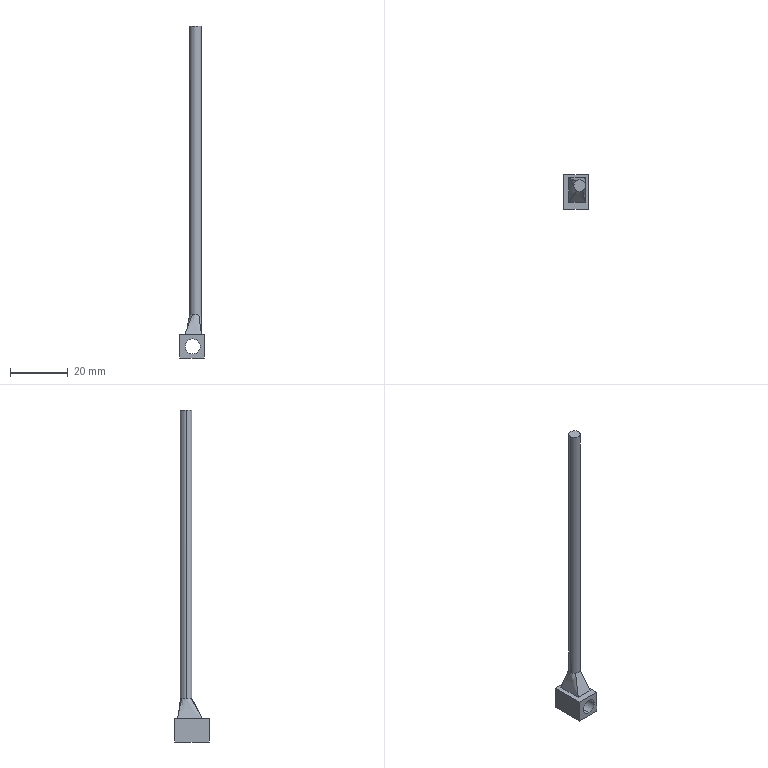Part | SolidWorks | features ICE 4, Blend 1, Extrusion 1 | 1 solid | 15 faces | box 8.5 x 12 x 115 mm | volume 2022 mm3 | plane 7 | cylinder 4 | spline 4 | commonest cylinder face diameters 4 x2 5.2 x2
STEP:
#1=CARTESIAN_POINT('',(-846.11,220.914,0.));
#2=VERTEX_POINT('',#1);
#3=CARTESIAN_POINT('',(-846.999,219.251,0.));
#4=VERTEX_POINT('',#3);
#5=CARTESIAN_POINT('',(-844.999,219.251,0.));
#6=DIRECTION('',(0.,0.,1.));
#7=DIRECTION('',(1.,0.,0.));
#8=AXIS2_PLACEMENT_3D('',#5,#6,#7);
#9=CIRCLE('',#8,2.);
#10=EDGE_CURVE('',#2,#4,#9,.T.);
#11=ORIENTED_EDGE('',*,*,#10,.T.);
#12=CARTESIAN_POINT('',(-846.999,219.251,100.));
#13=VERTEX_POINT('',#12);
#14=CARTESIAN_POINT('',(-846.999,219.251,-7.));
#15=DIRECTION('',(0.,0.,1.));
#16=VECTOR('',#15,1000.);
#17=LINE('',#14,#16);
#18=EDGE_CURVE('',#4,#13,#17,.T.);
#19=ORIENTED_EDGE('',*,*,#18,.T.);
#20=CARTESIAN_POINT('',(-842.999,219.251,100.));
#21=VERTEX_POINT('',#20);
#22=CARTESIAN_POINT('',(-844.999,219.251,100.));
#23=DIRECTION('',(0.,0.,1.));
#24=DIRECTION('',(1.,0.,0.));
#25=AXIS2_PLACEMENT_3D('',#22,#23,#24);
#26=CIRCLE('',#25,2.);
#27=EDGE_CURVE('',#21,#13,#26,.T.);
#28=ORIENTED_EDGE('',*,*,#27,.F.);
#29=CARTESIAN_POINT('',(-842.999,219.256,0.000005697));
#30=VERTEX_POINT('',#29);
#31=CARTESIAN_POINT('',(-842.999,219.251,-7.));
#32=DIRECTION('',(0.,0.,1.));
#33=VECTOR('',#32,1000.);
#34=LINE('',#31,#33);
#35=EDGE_CURVE('',#30,#21,#34,.T.);
#36=ORIENTED_EDGE('',*,*,#35,.F.);
#37=CARTESIAN_POINT('',(-843.888,220.914,0.));
#38=VERTEX_POINT('',#37);
#39=CARTESIAN_POINT('',(-843.888,220.914,0.));
#40=CARTESIAN_POINT('',(-843.866,220.899,0.));
#41=CARTESIAN_POINT('',(-843.84,220.881,-0.0001187));
#42=CARTESIAN_POINT('',(-843.796,220.849,-0.000475));
#43=CARTESIAN_POINT('',(-843.78,220.837,-0.0006234));
#44=CARTESIAN_POINT('',(-843.756,220.817,-0.0008905));
#45=CARTESIAN_POINT('',(-843.747,220.811,-0.000987));
#46=CARTESIAN_POINT('',(-843.73,220.797,-0.001195));
#47=CARTESIAN_POINT('',(-843.722,220.791,-0.001289));
#48=CARTESIAN_POINT('',(-843.671,220.747,-0.001968));
#49=CARTESIAN_POINT('',(-843.637,220.716,-0.0024));
#50=CARTESIAN_POINT('',(-843.598,220.678,-0.002883));
#51=CARTESIAN_POINT('',(-843.586,220.667,-0.003017));
#52=CARTESIAN_POINT('',(-843.572,220.652,-0.003175));
#53=CARTESIAN_POINT('',(-843.565,220.645,-0.003244));
#54=CARTESIAN_POINT('',(-843.558,220.638,-0.003307));
#55=CARTESIAN_POINT('',(-843.556,220.636,-0.00333));
#56=CARTESIAN_POINT('',(-843.554,220.634,-0.003344));
#57=CARTESIAN_POINT('',(-843.554,220.634,-0.003343));
#58=CARTESIAN_POINT('',(-843.526,220.604,-0.003576));
#59=CARTESIAN_POINT('',(-843.5,220.576,-0.003669));
#60=CARTESIAN_POINT('',(-843.453,220.52,-0.003607));
#61=CARTESIAN_POINT('',(-843.432,220.494,-0.003469));
#62=CARTESIAN_POINT('',(-843.388,220.436,-0.002871));
#63=CARTESIAN_POINT('',(-843.356,220.392,-0.002279));
#64=CARTESIAN_POINT('',(-843.32,220.338,-0.00134));
#65=CARTESIAN_POINT('',(-843.302,220.31,-0.0008085));
#66=CARTESIAN_POINT('',(-843.294,220.296,-0.000527));
#67=CARTESIAN_POINT('',(-843.29,220.29,-0.000403));
#68=CARTESIAN_POINT('',(-843.288,220.286,-0.0003196));
#69=CARTESIAN_POINT('',(-843.286,220.283,-0.000257));
#70=CARTESIAN_POINT('',(-843.284,220.28,-0.0001913));
#71=CARTESIAN_POINT('',(-843.282,220.277,-0.0001516));
#72=CARTESIAN_POINT('',(-843.278,220.269,-0.00008074));
#73=CARTESIAN_POINT('',(-843.274,220.262,-0.0000412));
#74=CARTESIAN_POINT('',(-843.266,220.25,0.0000152));
#75=CARTESIAN_POINT('',(-843.262,220.243,0.00001207));
#76=CARTESIAN_POINT('',(-843.252,220.225,-0.0001141));
#77=CARTESIAN_POINT('',(-843.245,220.212,-0.0002929));
#78=CARTESIAN_POINT('',(-843.239,220.201,-0.0005981));
#79=CARTESIAN_POINT('',(-843.235,220.193,-0.0008296));
#80=CARTESIAN_POINT('',(-843.233,220.191,-0.0009036));
#81=CARTESIAN_POINT('',(-843.225,220.175,-0.001502));
#82=CARTESIAN_POINT('',(-843.218,220.162,-0.002265));
#83=CARTESIAN_POINT('',(-843.212,220.148,-0.003443));
#84=CARTESIAN_POINT('',(-843.209,220.143,-0.004009));
#85=CARTESIAN_POINT('',(-843.207,220.139,-0.0044));
#86=CARTESIAN_POINT('',(-843.207,220.139,-0.004427));
#87=CARTESIAN_POINT('',(-843.194,220.113,-0.007893));
#88=CARTESIAN_POINT('',(-843.187,220.097,-0.0151));
#89=CARTESIAN_POINT('',(-843.182,220.086,-0.02857));
#90=CARTESIAN_POINT('',(-843.18,220.081,-0.03853));
#91=CARTESIAN_POINT('',(-843.178,220.077,-0.05581));
#92=CARTESIAN_POINT('',(-843.177,220.075,-0.06443));
#93=CARTESIAN_POINT('',(-843.176,220.074,-0.07044));
#94=CARTESIAN_POINT('',(-843.176,220.073,-0.07513));
#95=CARTESIAN_POINT('',(-843.175,220.072,-0.08376));
#96=CARTESIAN_POINT('',(-843.175,220.07,-0.09594));
#97=CARTESIAN_POINT('',(-843.174,220.068,-0.1133));
#98=CARTESIAN_POINT('',(-843.173,220.068,-0.1215));
#99=CARTESIAN_POINT('',(-843.173,220.067,-0.127));
#100=CARTESIAN_POINT('',(-843.173,220.067,-0.1312));
#101=CARTESIAN_POINT('',(-843.172,220.065,-0.146));
#102=CARTESIAN_POINT('',(-843.171,220.063,-0.17));
#103=CARTESIAN_POINT('',(-843.17,220.06,-0.2052));
#104=CARTESIAN_POINT('',(-843.169,220.058,-0.2246));
#105=CARTESIAN_POINT('',(-843.169,220.058,-0.2334));
#106=CARTESIAN_POINT('',(-843.169,220.057,-0.2392));
#107=CARTESIAN_POINT('',(-843.169,220.057,-0.2441));
#108=CARTESIAN_POINT('',(-843.167,220.054,-0.2815));
#109=CARTESIAN_POINT('',(-843.166,220.05,-0.3372));
#110=CARTESIAN_POINT('',(-843.162,220.042,-0.4498));
#111=CARTESIAN_POINT('',(-843.16,220.037,-0.5133));
#112=CARTESIAN_POINT('',(-843.157,220.031,-0.6002));
#113=CARTESIAN_POINT('',(-843.156,220.028,-0.6402));
#114=CARTESIAN_POINT('',(-843.155,220.026,-0.6674));
#115=CARTESIAN_POINT('',(-843.155,220.025,-0.6825));
#116=CARTESIAN_POINT('',(-843.142,219.994,-1.112));
#117=CARTESIAN_POINT('',(-843.131,219.966,-1.471));
#118=CARTESIAN_POINT('',(-843.118,219.931,-1.921));
#119=CARTESIAN_POINT('',(-843.114,219.92,-2.056));
#120=CARTESIAN_POINT('',(-843.109,219.905,-2.238));
#121=CARTESIAN_POINT('',(-843.107,219.898,-2.323));
#122=CARTESIAN_POINT('',(-843.104,219.891,-2.413));
#123=CARTESIAN_POINT('',(-843.103,219.887,-2.455));
#124=CARTESIAN_POINT('',(-843.102,219.886,-2.476));
#125=CARTESIAN_POINT('',(-843.102,219.885,-2.486));
#126=CARTESIAN_POINT('',(-843.102,219.884,-2.49));
#127=CARTESIAN_POINT('',(-843.102,219.884,-2.493));
#128=CARTESIAN_POINT('',(-843.102,219.884,-2.494));
#129=CARTESIAN_POINT('',(-843.092,219.855,-2.832));
#130=CARTESIAN_POINT('',(-843.084,219.827,-3.146));
#131=CARTESIAN_POINT('',(-843.072,219.786,-3.582));
#132=CARTESIAN_POINT('',(-843.068,219.771,-3.739));
#133=CARTESIAN_POINT('',(-843.064,219.755,-3.897));
#134=CARTESIAN_POINT('',(-843.063,219.752,-3.922));
#135=CARTESIAN_POINT('',(-843.062,219.751,-3.938));
#136=CARTESIAN_POINT('',(-843.062,219.749,-3.953));
#137=CARTESIAN_POINT('',(-843.06,219.742,-4.019));
#138=CARTESIAN_POINT('',(-843.056,219.726,-4.173));
#139=CARTESIAN_POINT('',(-843.042,219.668,-4.711));
#140=CARTESIAN_POINT('',(-843.032,219.617,-5.122));
#141=CARTESIAN_POINT('',(-843.022,219.557,-5.539));
#142=CARTESIAN_POINT('',(-843.018,219.528,-5.729));
#143=CARTESIAN_POINT('',(-843.014,219.495,-5.916));
#144=CARTESIAN_POINT('',(-843.012,219.479,-6.002));
#145=CARTESIAN_POINT('',(-843.011,219.471,-6.043));
#146=CARTESIAN_POINT('',(-843.011,219.467,-6.063));
#147=CARTESIAN_POINT('',(-843.01,219.465,-6.073));
#148=CARTESIAN_POINT('',(-843.01,219.464,-6.077));
#149=CARTESIAN_POINT('',(-843.01,219.463,-6.08));
#150=CARTESIAN_POINT('',(-843.01,219.463,-6.079));
#151=CARTESIAN_POINT('',(-843.008,219.441,-6.187));
#152=CARTESIAN_POINT('',(-843.006,219.42,-6.275));
#153=CARTESIAN_POINT('',(-843.004,219.39,-6.384));
#154=CARTESIAN_POINT('',(-843.003,219.375,-6.432));
#155=CARTESIAN_POINT('',(-843.002,219.358,-6.478));
#156=CARTESIAN_POINT('',(-843.001,219.349,-6.499));
#157=CARTESIAN_POINT('',(-843.001,219.345,-6.508));
#158=CARTESIAN_POINT('',(-843.001,219.343,-6.513));
#159=CARTESIAN_POINT('',(-843.001,219.342,-6.515));
#160=CARTESIAN_POINT('',(-843.001,219.342,-6.516));
#161=CARTESIAN_POINT('',(-843.001,219.342,-6.516));
#162=CARTESIAN_POINT('',(-843.,219.315,-6.572));
#163=CARTESIAN_POINT('',(-842.999,219.291,-6.599));
#164=CARTESIAN_POINT('',(-842.999,219.256,-6.597));
#165=CARTESIAN_POINT('',(-842.999,219.239,-6.586));
#166=CARTESIAN_POINT('',(-842.999,219.22,-6.555));
#167=CARTESIAN_POINT('',(-842.999,219.211,-6.535));
#168=CARTESIAN_POINT('',(-842.999,219.207,-6.525));
#169=CARTESIAN_POINT('',(-843.,219.205,-6.518));
#170=CARTESIAN_POINT('',(-843.,219.203,-6.513));
#171=CARTESIAN_POINT('',(-843.,219.193,-6.486));
#172=CARTESIAN_POINT('',(-843.,219.18,-6.44));
#173=CARTESIAN_POINT('',(-843.001,219.165,-6.371));
#174=CARTESIAN_POINT('',(-843.001,219.158,-6.333));
#175=CARTESIAN_POINT('',(-843.001,219.154,-6.313));
#176=CARTESIAN_POINT('',(-843.001,219.153,-6.304));
#177=CARTESIAN_POINT('',(-843.001,219.152,-6.298));
#178=CARTESIAN_POINT('',(-843.002,219.151,-6.294));
#179=CARTESIAN_POINT('',(-843.002,219.135,-6.197));
#180=CARTESIAN_POINT('',(-843.003,219.121,-6.075));
#181=CARTESIAN_POINT('',(-843.005,219.101,-5.851));
#182=CARTESIAN_POINT('',(-843.005,219.092,-5.728));
#183=CARTESIAN_POINT('',(-843.006,219.083,-5.568));
#184=CARTESIAN_POINT('',(-843.006,219.078,-5.483));
#185=CARTESIAN_POINT('',(-843.007,219.076,-5.439));
#186=CARTESIAN_POINT('',(-843.007,219.075,-5.417));
#187=CARTESIAN_POINT('',(-843.007,219.075,-5.408));
#188=CARTESIAN_POINT('',(-843.007,219.075,-5.401));
#189=CARTESIAN_POINT('',(-843.007,219.074,-5.397));
#190=CARTESIAN_POINT('',(-843.007,219.069,-5.278));
#191=CARTESIAN_POINT('',(-843.008,219.065,-5.145));
#192=CARTESIAN_POINT('',(-843.008,219.059,-4.92));
#193=CARTESIAN_POINT('',(-843.008,219.057,-4.801));
#194=CARTESIAN_POINT('',(-843.009,219.055,-4.652));
#195=CARTESIAN_POINT('',(-843.009,219.054,-4.575));
#196=CARTESIAN_POINT('',(-843.009,219.054,-4.535));
#197=CARTESIAN_POINT('',(-843.009,219.054,-4.515));
#198=CARTESIAN_POINT('',(-843.009,219.054,-4.507));
#199=CARTESIAN_POINT('',(-843.009,219.054,-4.501));
#200=CARTESIAN_POINT('',(-843.009,219.054,-4.497));
#201=CARTESIAN_POINT('',(-843.009,219.053,-4.402));
#202=CARTESIAN_POINT('',(-843.009,219.053,-4.28));
#203=CARTESIAN_POINT('',(-843.009,219.054,-4.055));
#204=CARTESIAN_POINT('',(-843.009,219.054,-3.973));
#205=CARTESIAN_POINT('',(-843.009,219.056,-3.839));
#206=CARTESIAN_POINT('',(-843.008,219.057,-3.769));
#207=CARTESIAN_POINT('',(-843.008,219.058,-3.696));
#208=CARTESIAN_POINT('',(-843.008,219.059,-3.646));
#209=CARTESIAN_POINT('',(-843.008,219.059,-3.619));
#210=CARTESIAN_POINT('',(-843.008,219.067,-3.208));
#211=CARTESIAN_POINT('',(-843.006,219.078,-2.864));
#212=CARTESIAN_POINT('',(-843.005,219.096,-2.414));
#213=CARTESIAN_POINT('',(-843.005,219.102,-2.275));
#214=CARTESIAN_POINT('',(-843.004,219.112,-2.083));
#215=CARTESIAN_POINT('',(-843.004,219.117,-1.991));
#216=CARTESIAN_POINT('',(-843.003,219.122,-1.891));
#217=CARTESIAN_POINT('',(-843.003,219.125,-1.842));
#218=CARTESIAN_POINT('',(-843.003,219.126,-1.819));
#219=CARTESIAN_POINT('',(-843.003,219.127,-1.809));
#220=CARTESIAN_POINT('',(-843.003,219.127,-1.802));
#221=CARTESIAN_POINT('',(-843.003,219.127,-1.8));
#222=CARTESIAN_POINT('',(-843.001,219.161,-1.196));
#223=CARTESIAN_POINT('',(-842.999,219.205,-0.5978));
#224=CARTESIAN_POINT('',(-842.999,219.256,0.000005697));
#225=B_SPLINE_CURVE_WITH_KNOTS('',3,(#39,#40,#41,#42,#43,#44,#45,#46,#47,#48,#49,#50,#51,#52,#53,#54,#55,#56,#57,#58,#59,#60,#61,#62,#63,#64,#65,#66,#67,#68,#69,#70,#71,#72,#73,#74,#75,#76,#77,#78,#79,#80,#81,#82,#83,#84,#85,#86,#87,#88,#89,#90,#91,#92,#93,#94,#95,#96,#97,#98,#99,#100,#101,#102,#103,#104,#105,#106,#107,#108,#109,#110,#111,#112,#113,#114,#115,#116,#117,#118,#119,#120,#121,#122,#123,#124,#125,#126,#127,#128,#129,#130,#131,#132,#133,#134,#135,#136,#137,#138,#139,#140,#141,#142,#143,#144,#145,#146,#147,#148,#149,#150,#151,#152,#153,#154,#155,#156,#157,#158,#159,#160,#161,#162,#163,#164,#165,#166,#167,#168,#169,#170,#171,#172,#173,#174,#175,#176,#177,#178,#179,#180,#181,#182,#183,#184,#185,#186,#187,#188,#189,#190,#191,#192,#193,#194,#195,#196,#197,#198,#199,#200,#201,#202,#203,#204,#205,#206,#207,#208,#209,#210,#211,#212,#213,#214,#215,#216,#217,#218,#219,#220,#221,#222,#223,#224),.UNSPECIFIED.,.F.,.F.,(4,2,2,2,2,2,2,1,1,2,2,2,2,1,1,1,1,2,2,2,2,2,1,2,2,1,1,2,2,2,1,1,2,2,1,1,2,2,1,1,1,2,2,2,1,1,2,2,2,2,1,1,1,1,1,2,2,2,1,1,2,2,1,1,2,1,1,1,1,1,1,2,2,2,1,1,1,1,1,2,2,2,1,1,1,2,2,1,1,1,1,2,2,2,1,1,1,1,1,2,2,2,1,1,1,1,1,2,2,2,2,1,2,2,2,2,1,1,1,1,2,2,4),(0.,0.007813,0.01172,0.01367,0.01563,0.02344,0.02734,0.0293,0.03027,0.03076,0.03125,0.03906,0.04688,0.05469,0.05859,0.06055,0.06152,0.06201,0.0625,0.06348,0.06445,0.06641,0.06836,0.06934,0.07031,0.07227,0.07324,0.07373,0.07422,0.07813,0.08008,0.08105,0.08154,0.08203,0.08398,0.08496,0.08545,0.08594,0.08984,0.0918,0.09277,0.09326,0.09375,0.1094,0.1172,0.1211,0.123,0.125,0.1875,0.2188,0.2344,0.2422,0.2461,0.248,0.249,0.2495,0.25,0.3125,0.3438,0.3477,0.3496,0.3516,0.3594,0.375,0.4375,0.4688,0.4844,0.4922,0.4961,0.498,0.499,0.4995,0.5,0.5156,0.5234,0.5273,0.5293,0.5303,0.5308,0.531,0.5313,0.5391,0.543,0.5449,0.5459,0.5464,0.5469,0.5547,0.5586,0.5605,0.5615,0.562,0.5625,0.5938,0.6094,0.6172,0.6211,0.623,0.624,0.6245,0.625,0.6563,0.6719,0.6797,0.6836,0.6855,0.6865,0.687,0.6875,0.7188,0.7344,0.7422,0.7461,0.75,0.8125,0.8438,0.8594,0.8672,0.8711,0.873,0.874,0.875,1.),.UNSPECIFIED.);
#226=EDGE_CURVE('',#38,#30,#225,.T.);
#227=ORIENTED_EDGE('',*,*,#226,.F.);
#228=CARTESIAN_POINT('',(-844.999,219.251,0.));
#229=DIRECTION('',(0.,0.,1.));
#230=DIRECTION('',(1.,0.,0.));
#231=AXIS2_PLACEMENT_3D('',#228,#229,#230);
#232=CIRCLE('',#231,2.);
#233=EDGE_CURVE('',#38,#2,#232,.T.);
#234=ORIENTED_EDGE('',*,*,#233,.T.);
#235=EDGE_LOOP('',(#11,#19,#28,#36,#227,#234));
#236=FACE_OUTER_BOUND('',#235,.T.);
#237=CARTESIAN_POINT('',(-844.999,219.251,-7.));
#238=DIRECTION('',(0.,0.,1.));
#239=DIRECTION('',(1.,0.,0.));
#240=AXIS2_PLACEMENT_3D('',#237,#238,#239);
#241=CYLINDRICAL_SURFACE('',#240,2.);
#242=ADVANCED_FACE('',(#236),#241,.T.);
#243=CARTESIAN_POINT('',(-845.999,211.251,-8.4));
#244=VERTEX_POINT('',#243);
#245=CARTESIAN_POINT('',(-845.999,211.251,-13.6));
#246=VERTEX_POINT('',#245);
#247=CARTESIAN_POINT('',(-845.999,211.251,-11.));
#248=DIRECTION('',(0.,-1.,0.));
#249=DIRECTION('',(0.,0.,-1.));
#250=AXIS2_PLACEMENT_3D('',#247,#248,#249);
#251=CIRCLE('',#250,2.6);
#252=EDGE_CURVE('',#244,#246,#251,.T.);
#253=ORIENTED_EDGE('',*,*,#252,.T.);
#254=CARTESIAN_POINT('',(-845.999,223.251,-13.6));
#255=VERTEX_POINT('',#254);
#256=CARTESIAN_POINT('',(-845.999,215.251,-13.6));
#257=DIRECTION('',(0.,1.,0.));
#258=VECTOR('',#257,1000.);
#259=LINE('',#256,#258);
#260=EDGE_CURVE('',#246,#255,#259,.T.);
#261=ORIENTED_EDGE('',*,*,#260,.T.);
#262=CARTESIAN_POINT('',(-845.999,223.251,-8.4));
#263=VERTEX_POINT('',#262);
#264=CARTESIAN_POINT('',(-845.999,223.251,-11.));
#265=DIRECTION('',(0.,1.,0.));
#266=DIRECTION('',(0.,0.,1.));
#267=AXIS2_PLACEMENT_3D('',#264,#265,#266);
#268=CIRCLE('',#267,2.6);
#269=EDGE_CURVE('',#255,#263,#268,.T.);
#270=ORIENTED_EDGE('',*,*,#269,.T.);
#271=CARTESIAN_POINT('',(-845.999,215.251,-8.4));
#272=DIRECTION('',(0.,1.,0.));
#273=VECTOR('',#272,1000.);
#274=LINE('',#271,#273);
#275=EDGE_CURVE('',#244,#263,#274,.T.);
#276=ORIENTED_EDGE('',*,*,#275,.F.);
#277=EDGE_LOOP('',(#253,#261,#270,#276));
#278=FACE_OUTER_BOUND('',#277,.T.);
#279=CARTESIAN_POINT('',(-845.999,215.251,-11.));
#280=DIRECTION('',(0.,1.,0.));
#281=DIRECTION('',(0.,0.,1.));
#282=AXIS2_PLACEMENT_3D('',#279,#280,#281);
#283=CYLINDRICAL_SURFACE('',#282,2.6);
#284=ADVANCED_FACE('',(#278),#283,.F.);
#285=CARTESIAN_POINT('',(-841.999,223.251,-7.));
#286=VERTEX_POINT('',#285);
#287=CARTESIAN_POINT('',(-841.999,211.251,-7.));
#288=VERTEX_POINT('',#287);
#289=CARTESIAN_POINT('',(-841.999,215.251,-7.));
#290=DIRECTION('',(0.,-1.,0.));
#291=VECTOR('',#290,1000.);
#292=LINE('',#289,#291);
#293=EDGE_CURVE('',#286,#288,#292,.T.);
#294=ORIENTED_EDGE('',*,*,#293,.T.);
#295=CARTESIAN_POINT('',(-841.999,211.251,-15.));
#296=VERTEX_POINT('',#295);
#297=CARTESIAN_POINT('',(-841.999,211.251,-15.));
#298=DIRECTION('',(0.,0.,1.));
#299=VECTOR('',#298,1000.);
#300=LINE('',#297,#299);
#301=EDGE_CURVE('',#296,#288,#300,.T.);
#302=ORIENTED_EDGE('',*,*,#301,.F.);
#303=CARTESIAN_POINT('',(-841.999,223.251,-15.));
#304=VERTEX_POINT('',#303);
#305=CARTESIAN_POINT('',(-841.999,215.251,-15.));
#306=DIRECTION('',(0.,-1.,0.));
#307=VECTOR('',#306,1000.);
#308=LINE('',#305,#307);
#309=EDGE_CURVE('',#304,#296,#308,.T.);
#310=ORIENTED_EDGE('',*,*,#309,.F.);
#311=CARTESIAN_POINT('',(-841.999,223.251,-15.));
#312=DIRECTION('',(0.,0.,1.));
#313=VECTOR('',#312,1000.);
#314=LINE('',#311,#313);
#315=EDGE_CURVE('',#304,#286,#314,.T.);
#316=ORIENTED_EDGE('',*,*,#315,.T.);
#317=EDGE_LOOP('',(#294,#302,#310,#316));
#318=FACE_OUTER_BOUND('',#317,.T.);
#319=CARTESIAN_POINT('',(-841.999,215.251,-15.));
#320=DIRECTION('',(-1.,0.,0.));
#321=DIRECTION('',(0.,0.,1.));
#322=AXIS2_PLACEMENT_3D('',#319,#320,#321);
#323=PLANE('',#322);
#324=ADVANCED_FACE('',(#318),#323,.F.);
#325=CARTESIAN_POINT('',(-845.999,223.251,-11.));
#326=DIRECTION('',(0.,1.,0.));
#327=DIRECTION('',(0.,0.,1.));
#328=AXIS2_PLACEMENT_3D('',#325,#326,#327);
#329=CIRCLE('',#328,2.6);
#330=EDGE_CURVE('',#263,#255,#329,.T.);
#331=ORIENTED_EDGE('',*,*,#330,.F.);
#332=ORIENTED_EDGE('',*,*,#269,.F.);
#333=EDGE_LOOP('',(#331,#332));
#334=FACE_BOUND('',#333,.T.);
#335=CARTESIAN_POINT('',(-850.499,223.251,-7.));
#336=VERTEX_POINT('',#335);
#337=CARTESIAN_POINT('',(-849.999,223.251,-7.));
#338=DIRECTION('',(1.,0.,0.));
#339=VECTOR('',#338,1000.);
#340=LINE('',#337,#339);
#341=EDGE_CURVE('',#336,#286,#340,.T.);
#342=ORIENTED_EDGE('',*,*,#341,.T.);
#343=ORIENTED_EDGE('',*,*,#315,.F.);
#344=CARTESIAN_POINT('',(-850.499,223.251,-15.));
#345=VERTEX_POINT('',#344);
#346=CARTESIAN_POINT('',(-849.999,223.251,-15.));
#347=DIRECTION('',(1.,0.,0.));
#348=VECTOR('',#347,1000.);
#349=LINE('',#346,#348);
#350=EDGE_CURVE('',#345,#304,#349,.T.);
#351=ORIENTED_EDGE('',*,*,#350,.F.);
#352=CARTESIAN_POINT('',(-850.499,223.251,-7.));
#353=DIRECTION('',(0.,0.,-1.));
#354=VECTOR('',#353,1000.);
#355=LINE('',#352,#354);
#356=EDGE_CURVE('',#336,#345,#355,.T.);
#357=ORIENTED_EDGE('',*,*,#356,.F.);
#358=EDGE_LOOP('',(#342,#343,#351,#357));
#359=FACE_OUTER_BOUND('',#358,.T.);
#360=CARTESIAN_POINT('',(-849.999,223.251,-15.));
#361=DIRECTION('',(0.,-1.,0.));
#362=DIRECTION('',(0.,0.,-1.));
#363=AXIS2_PLACEMENT_3D('',#360,#361,#362);
#364=PLANE('',#363);
#365=ADVANCED_FACE('',(#334,#359),#364,.F.);
#366=ORIENTED_EDGE('',*,*,#309,.T.);
#367=CARTESIAN_POINT('',(-850.499,211.251,-15.));
#368=VERTEX_POINT('',#367);
#369=CARTESIAN_POINT('',(-850.499,211.251,-15.));
#370=DIRECTION('',(1.,0.,0.));
#371=VECTOR('',#370,1000.);
#372=LINE('',#369,#371);
#373=EDGE_CURVE('',#368,#296,#372,.T.);
#374=ORIENTED_EDGE('',*,*,#373,.F.);
#375=CARTESIAN_POINT('',(-850.499,223.251,-15.));
#376=DIRECTION('',(0.,-1.,0.));
#377=VECTOR('',#376,1000.);
#378=LINE('',#375,#377);
#379=EDGE_CURVE('',#345,#368,#378,.T.);
#380=ORIENTED_EDGE('',*,*,#379,.F.);
#381=ORIENTED_EDGE('',*,*,#350,.T.);
#382=EDGE_LOOP('',(#366,#374,#380,#381));
#383=FACE_OUTER_BOUND('',#382,.T.);
#384=CARTESIAN_POINT('',(0.,0.,-15.));
#385=DIRECTION('',(0.,0.,-1.));
#386=DIRECTION('',(-1.,0.,0.));
#387=AXIS2_PLACEMENT_3D('',#384,#385,#386);
#388=PLANE('',#387);
#389=ADVANCED_FACE('',(#383),#388,.T.);
#390=CARTESIAN_POINT('',(-848.75,213.628,-7.));
#391=VERTEX_POINT('',#390);
#392=CARTESIAN_POINT('',(-842.993,213.628,-7.));
#393=VERTEX_POINT('',#392);
#394=CARTESIAN_POINT('',(-848.75,213.628,-7.));
#395=DIRECTION('',(1.,0.,0.));
#396=VECTOR('',#395,1000.);
#397=LINE('',#394,#396);
#398=EDGE_CURVE('',#391,#393,#397,.T.);
#399=ORIENTED_EDGE('',*,*,#398,.F.);
#400=CARTESIAN_POINT('',(-848.75,222.246,-7.));
#401=VERTEX_POINT('',#400);
#402=CARTESIAN_POINT('',(-848.75,222.246,-7.));
#403=DIRECTION('',(0.,-1.,0.));
#404=VECTOR('',#403,1000.);
#405=LINE('',#402,#404);
#406=EDGE_CURVE('',#401,#391,#405,.T.);
#407=ORIENTED_EDGE('',*,*,#406,.F.);
#408=CARTESIAN_POINT('',(-842.993,222.246,-7.));
#409=VERTEX_POINT('',#408);
#410=CARTESIAN_POINT('',(-842.993,222.246,-7.));
#411=DIRECTION('',(-1.,0.,0.));
#412=VECTOR('',#411,1000.);
#413=LINE('',#410,#412);
#414=EDGE_CURVE('',#409,#401,#413,.T.);
#415=ORIENTED_EDGE('',*,*,#414,.F.);
#416=CARTESIAN_POINT('',(-842.993,213.628,-7.));
#417=DIRECTION('',(0.,1.,0.));
#418=VECTOR('',#417,1000.);
#419=LINE('',#416,#418);
#420=EDGE_CURVE('',#393,#409,#419,.T.);
#421=ORIENTED_EDGE('',*,*,#420,.F.);
#422=EDGE_LOOP('',(#399,#407,#415,#421));
#423=FACE_BOUND('',#422,.T.);
#424=ORIENTED_EDGE('',*,*,#293,.F.);
#425=ORIENTED_EDGE('',*,*,#341,.F.);
#426=CARTESIAN_POINT('',(-850.499,211.251,-7.));
#427=VERTEX_POINT('',#426);
#428=CARTESIAN_POINT('',(-850.499,215.251,-7.));
#429=DIRECTION('',(0.,1.,0.));
#430=VECTOR('',#429,1000.);
#431=LINE('',#428,#430);
#432=EDGE_CURVE('',#427,#336,#431,.T.);
#433=ORIENTED_EDGE('',*,*,#432,.F.);
#434=CARTESIAN_POINT('',(-841.999,211.251,-7.));
#435=DIRECTION('',(-1.,0.,0.));
#436=VECTOR('',#435,1000.);
#437=LINE('',#434,#436);
#438=EDGE_CURVE('',#288,#427,#437,.T.);
#439=ORIENTED_EDGE('',*,*,#438,.F.);
#440=EDGE_LOOP('',(#424,#425,#433,#439));
#441=FACE_OUTER_BOUND('',#440,.T.);
#442=CARTESIAN_POINT('',(0.,0.,-7.));
#443=DIRECTION('',(0.,0.,-1.));
#444=DIRECTION('',(-1.,0.,0.));
#445=AXIS2_PLACEMENT_3D('',#442,#443,#444);
#446=PLANE('',#445);
#447=ADVANCED_FACE('',(#423,#441),#446,.F.);
#448=ORIENTED_EDGE('',*,*,#260,.F.);
#449=CARTESIAN_POINT('',(-845.999,211.251,-11.));
#450=DIRECTION('',(0.,-1.,0.));
#451=DIRECTION('',(0.,0.,-1.));
#452=AXIS2_PLACEMENT_3D('',#449,#450,#451);
#453=CIRCLE('',#452,2.6);
#454=EDGE_CURVE('',#246,#244,#453,.T.);
#455=ORIENTED_EDGE('',*,*,#454,.T.);
#456=ORIENTED_EDGE('',*,*,#275,.T.);
#457=ORIENTED_EDGE('',*,*,#330,.T.);
#458=EDGE_LOOP('',(#448,#455,#456,#457));
#459=FACE_OUTER_BOUND('',#458,.T.);
#460=CARTESIAN_POINT('',(-845.999,215.251,-11.));
#461=DIRECTION('',(0.,1.,0.));
#462=DIRECTION('',(0.,0.,1.));
#463=AXIS2_PLACEMENT_3D('',#460,#461,#462);
#464=CYLINDRICAL_SURFACE('',#463,2.6);
#465=ADVANCED_FACE('',(#459),#464,.F.);
#466=ORIENTED_EDGE('',*,*,#379,.T.);
#467=CARTESIAN_POINT('',(-850.499,211.251,-7.));
#468=DIRECTION('',(0.,0.,-1.));
#469=VECTOR('',#468,1000.);
#470=LINE('',#467,#469);
#471=EDGE_CURVE('',#427,#368,#470,.T.);
#472=ORIENTED_EDGE('',*,*,#471,.F.);
#473=ORIENTED_EDGE('',*,*,#432,.T.);
#474=ORIENTED_EDGE('',*,*,#356,.T.);
#475=EDGE_LOOP('',(#466,#472,#473,#474));
#476=FACE_OUTER_BOUND('',#475,.T.);
#477=CARTESIAN_POINT('',(-850.499,0.,0.));
#478=DIRECTION('',(-1.,0.,0.));
#479=DIRECTION('',(0.,0.,1.));
#480=AXIS2_PLACEMENT_3D('',#477,#478,#479);
#481=PLANE('',#480);
#482=ADVANCED_FACE('',(#476),#481,.T.);
#483=ORIENTED_EDGE('',*,*,#301,.T.);
#484=ORIENTED_EDGE('',*,*,#438,.T.);
#485=ORIENTED_EDGE('',*,*,#471,.T.);
#486=ORIENTED_EDGE('',*,*,#373,.T.);
#487=EDGE_LOOP('',(#483,#484,#485,#486));
#488=FACE_OUTER_BOUND('',#487,.T.);
#489=ORIENTED_EDGE('',*,*,#252,.F.);
#490=ORIENTED_EDGE('',*,*,#454,.F.);
#491=EDGE_LOOP('',(#489,#490));
#492=FACE_BOUND('',#491,.T.);
#493=CARTESIAN_POINT('',(0.,211.251,0.));
#494=DIRECTION('',(0.,-1.,0.));
#495=DIRECTION('',(0.,0.,-1.));
#496=AXIS2_PLACEMENT_3D('',#493,#494,#495);
#497=PLANE('',#496);
#498=ADVANCED_FACE('',(#488,#492),#497,.T.);
#499=CARTESIAN_POINT('',(-843.441,221.58,-3.5));
#500=DIRECTION('',(-0.1246,-0.1855,0.9747));
#501=VECTOR('',#500,1000.);
#502=LINE('',#499,#501);
#503=EDGE_CURVE('',#409,#38,#502,.T.);
#504=ORIENTED_EDGE('',*,*,#503,.T.);
#505=ORIENTED_EDGE('',*,*,#226,.T.);
#506=CARTESIAN_POINT('',(-843.888,217.588,0.));
#507=VERTEX_POINT('',#506);
#508=CARTESIAN_POINT('',(-844.999,219.251,0.));
#509=DIRECTION('',(0.,0.,1.));
#510=DIRECTION('',(1.,0.,0.));
#511=AXIS2_PLACEMENT_3D('',#508,#509,#510);
#512=CIRCLE('',#511,2.);
#513=EDGE_CURVE('',#507,#30,#512,.T.);
#514=ORIENTED_EDGE('',*,*,#513,.F.);
#515=CARTESIAN_POINT('',(-843.441,215.608,-3.5));
#516=DIRECTION('',(0.1106,-0.4894,-0.865));
#517=VECTOR('',#516,1000.);
#518=LINE('',#515,#517);
#519=EDGE_CURVE('',#507,#393,#518,.T.);
#520=ORIENTED_EDGE('',*,*,#519,.T.);
#521=ORIENTED_EDGE('',*,*,#420,.T.);
#522=EDGE_LOOP('',(#504,#505,#514,#520,#521));
#523=FACE_OUTER_BOUND('',#522,.T.);
#524=CARTESIAN_POINT('',(-843.888,220.914,0.));
#525=CARTESIAN_POINT('',(-842.993,222.246,-7.));
#526=CARTESIAN_POINT('',(-843.658,220.76,0.));
#527=CARTESIAN_POINT('',(-842.993,221.528,-7.));
#528=CARTESIAN_POINT('',(-843.432,220.537,0.));
#529=CARTESIAN_POINT('',(-842.993,220.81,-7.));
#530=CARTESIAN_POINT('',(-843.183,220.105,0.));
#531=CARTESIAN_POINT('',(-842.993,219.733,-7.));
#532=CARTESIAN_POINT('',(-843.115,219.945,0.));
#533=CARTESIAN_POINT('',(-842.993,219.373,-7.));
#534=CARTESIAN_POINT('',(-843.023,219.607,0.));
#535=CARTESIAN_POINT('',(-842.993,218.655,-7.));
#536=CARTESIAN_POINT('',(-842.999,219.429,0.));
#537=CARTESIAN_POINT('',(-842.993,218.296,-7.));
#538=CARTESIAN_POINT('',(-842.999,219.073,0.));
#539=CARTESIAN_POINT('',(-842.993,217.578,-7.));
#540=CARTESIAN_POINT('',(-843.023,218.895,0.));
#541=CARTESIAN_POINT('',(-842.993,217.219,-7.));
#542=CARTESIAN_POINT('',(-843.115,218.557,0.));
#543=CARTESIAN_POINT('',(-842.993,216.501,-7.));
#544=CARTESIAN_POINT('',(-843.183,218.397,0.));
#545=CARTESIAN_POINT('',(-842.993,216.142,-7.));
#546=CARTESIAN_POINT('',(-843.432,217.965,0.));
#547=CARTESIAN_POINT('',(-842.993,215.064,-7.));
#548=CARTESIAN_POINT('',(-843.658,217.742,0.));
#549=CARTESIAN_POINT('',(-842.993,214.346,-7.));
#550=CARTESIAN_POINT('',(-843.888,217.588,0.));
#551=CARTESIAN_POINT('',(-842.993,213.628,-7.));
#552=B_SPLINE_SURFACE_WITH_KNOTS('',3,1,((#524,#525),(#526,#527),(#528,#529),(#530,#531),(#532,#533),(#534,#535),(#536,#537),(#538,#539),(#540,#541),(#542,#543),(#544,#545),(#546,#547),(#548,#549),(#550,#551)),.UNSPECIFIED.,.F.,.F.,.F.,(4,2,2,2,2,2,4),(2,2),(0.,0.25,0.375,0.5,0.625,0.75,1.),(0.,1.),.UNSPECIFIED.);
#553=ADVANCED_FACE('',(#523),#552,.T.);
#554=CARTESIAN_POINT('',(-846.11,217.588,0.));
#555=VERTEX_POINT('',#554);
#556=CARTESIAN_POINT('',(-844.999,219.251,0.));
#557=DIRECTION('',(0.,0.,1.));
#558=DIRECTION('',(1.,0.,0.));
#559=AXIS2_PLACEMENT_3D('',#556,#557,#558);
#560=CIRCLE('',#559,2.);
#561=EDGE_CURVE('',#555,#507,#560,.T.);
#562=ORIENTED_EDGE('',*,*,#561,.F.);
#563=CARTESIAN_POINT('',(-847.43,215.608,-3.5));
#564=DIRECTION('',(-0.3119,-0.4678,-0.827));
#565=VECTOR('',#564,1000.);
#566=LINE('',#563,#565);
#567=EDGE_CURVE('',#555,#391,#566,.T.);
#568=ORIENTED_EDGE('',*,*,#567,.T.);
#569=ORIENTED_EDGE('',*,*,#398,.T.);
#570=ORIENTED_EDGE('',*,*,#519,.F.);
#571=EDGE_LOOP('',(#562,#568,#569,#570));
#572=FACE_OUTER_BOUND('',#571,.T.);
#573=CARTESIAN_POINT('',(-843.888,217.588,0.));
#574=CARTESIAN_POINT('',(-842.993,213.628,-7.));
#575=CARTESIAN_POINT('',(-844.042,217.485,0.));
#576=CARTESIAN_POINT('',(-843.473,213.628,-7.));
#577=CARTESIAN_POINT('',(-844.217,217.399,0.));
#578=CARTESIAN_POINT('',(-843.952,213.628,-7.));
#579=CARTESIAN_POINT('',(-844.595,217.282,0.));
#580=CARTESIAN_POINT('',(-844.912,213.628,-7.));
#581=CARTESIAN_POINT('',(-844.797,217.251,0.));
#582=CARTESIAN_POINT('',(-845.392,213.628,-7.));
#583=CARTESIAN_POINT('',(-845.201,217.251,0.));
#584=CARTESIAN_POINT('',(-846.351,213.628,-7.));
#585=CARTESIAN_POINT('',(-845.403,217.282,0.));
#586=CARTESIAN_POINT('',(-846.831,213.628,-7.));
#587=CARTESIAN_POINT('',(-845.781,217.399,0.));
#588=CARTESIAN_POINT('',(-847.79,213.628,-7.));
#589=CARTESIAN_POINT('',(-845.956,217.485,0.));
#590=CARTESIAN_POINT('',(-848.27,213.628,-7.));
#591=CARTESIAN_POINT('',(-846.11,217.588,0.));
#592=CARTESIAN_POINT('',(-848.75,213.628,-7.));
#593=B_SPLINE_SURFACE_WITH_KNOTS('',3,1,((#573,#574),(#575,#576),(#577,#578),(#579,#580),(#581,#582),(#583,#584),(#585,#586),(#587,#588),(#589,#590),(#591,#592)),.UNSPECIFIED.,.F.,.F.,.F.,(4,2,2,2,4),(2,2),(0.,0.25,0.5,0.75,1.),(0.,1.),.UNSPECIFIED.);
#594=ADVANCED_FACE('',(#572),#593,.T.);
#595=ORIENTED_EDGE('',*,*,#233,.F.);
#596=ORIENTED_EDGE('',*,*,#503,.F.);
#597=ORIENTED_EDGE('',*,*,#414,.T.);
#598=CARTESIAN_POINT('',(-847.43,221.58,-3.5));
#599=DIRECTION('',(-0.3474,0.1753,-0.9212));
#600=VECTOR('',#599,1000.);
#601=LINE('',#598,#600);
#602=EDGE_CURVE('',#2,#401,#601,.T.);
#603=ORIENTED_EDGE('',*,*,#602,.F.);
#604=EDGE_LOOP('',(#595,#596,#597,#603));
#605=FACE_OUTER_BOUND('',#604,.T.);
#606=CARTESIAN_POINT('',(-846.11,220.914,0.));
#607=CARTESIAN_POINT('',(-848.75,222.246,-7.));
#608=CARTESIAN_POINT('',(-845.956,221.017,0.));
#609=CARTESIAN_POINT('',(-848.27,222.246,-7.));
#610=CARTESIAN_POINT('',(-845.781,221.102,0.));
#611=CARTESIAN_POINT('',(-847.79,222.246,-7.));
#612=CARTESIAN_POINT('',(-845.403,221.22,0.));
#613=CARTESIAN_POINT('',(-846.831,222.246,-7.));
#614=CARTESIAN_POINT('',(-845.201,221.251,0.));
#615=CARTESIAN_POINT('',(-846.351,222.246,-7.));
#616=CARTESIAN_POINT('',(-844.797,221.251,0.));
#617=CARTESIAN_POINT('',(-845.392,222.246,-7.));
#618=CARTESIAN_POINT('',(-844.595,221.22,0.));
#619=CARTESIAN_POINT('',(-844.912,222.246,-7.));
#620=CARTESIAN_POINT('',(-844.217,221.102,0.));
#621=CARTESIAN_POINT('',(-843.952,222.246,-7.));
#622=CARTESIAN_POINT('',(-844.042,221.017,0.));
#623=CARTESIAN_POINT('',(-843.473,222.246,-7.));
#624=CARTESIAN_POINT('',(-843.888,220.914,0.));
#625=CARTESIAN_POINT('',(-842.993,222.246,-7.));
#626=B_SPLINE_SURFACE_WITH_KNOTS('',3,1,((#606,#607),(#608,#609),(#610,#611),(#612,#613),(#614,#615),(#616,#617),(#618,#619),(#620,#621),(#622,#623),(#624,#625)),.UNSPECIFIED.,.F.,.F.,.F.,(4,2,2,2,4),(2,2),(0.,0.25,0.5,0.75,1.),(0.,1.),.UNSPECIFIED.);
#627=ADVANCED_FACE('',(#605),#626,.T.);
#628=ORIENTED_EDGE('',*,*,#10,.F.);
#629=ORIENTED_EDGE('',*,*,#602,.T.);
#630=ORIENTED_EDGE('',*,*,#406,.T.);
#631=ORIENTED_EDGE('',*,*,#567,.F.);
#632=CARTESIAN_POINT('',(-844.999,219.251,0.));
#633=DIRECTION('',(0.,0.,1.));
#634=DIRECTION('',(1.,0.,0.));
#635=AXIS2_PLACEMENT_3D('',#632,#633,#634);
#636=CIRCLE('',#635,2.);
#637=EDGE_CURVE('',#4,#555,#636,.T.);
#638=ORIENTED_EDGE('',*,*,#637,.F.);
#639=EDGE_LOOP('',(#628,#629,#630,#631,#638));
#640=FACE_OUTER_BOUND('',#639,.T.);
#641=CARTESIAN_POINT('',(-846.11,217.588,0.));
#642=CARTESIAN_POINT('',(-848.75,213.628,-7.));
#643=CARTESIAN_POINT('',(-846.34,217.742,0.));
#644=CARTESIAN_POINT('',(-848.75,214.346,-7.));
#645=CARTESIAN_POINT('',(-846.566,217.965,0.));
#646=CARTESIAN_POINT('',(-848.75,215.064,-7.));
#647=CARTESIAN_POINT('',(-846.815,218.397,0.));
#648=CARTESIAN_POINT('',(-848.75,216.142,-7.));
#649=CARTESIAN_POINT('',(-846.883,218.557,0.));
#650=CARTESIAN_POINT('',(-848.75,216.501,-7.));
#651=CARTESIAN_POINT('',(-846.975,218.895,0.));
#652=CARTESIAN_POINT('',(-848.75,217.219,-7.));
#653=CARTESIAN_POINT('',(-846.999,219.073,0.));
#654=CARTESIAN_POINT('',(-848.75,217.578,-7.));
#655=CARTESIAN_POINT('',(-846.999,219.429,0.));
#656=CARTESIAN_POINT('',(-848.75,218.296,-7.));
#657=CARTESIAN_POINT('',(-846.975,219.607,0.));
#658=CARTESIAN_POINT('',(-848.75,218.655,-7.));
#659=CARTESIAN_POINT('',(-846.883,219.945,0.));
#660=CARTESIAN_POINT('',(-848.75,219.373,-7.));
#661=CARTESIAN_POINT('',(-846.815,220.105,0.));
#662=CARTESIAN_POINT('',(-848.75,219.733,-7.));
#663=CARTESIAN_POINT('',(-846.566,220.537,0.));
#664=CARTESIAN_POINT('',(-848.75,220.81,-7.));
#665=CARTESIAN_POINT('',(-846.34,220.76,0.));
#666=CARTESIAN_POINT('',(-848.75,221.528,-7.));
#667=CARTESIAN_POINT('',(-846.11,220.914,0.));
#668=CARTESIAN_POINT('',(-848.75,222.246,-7.));
#669=B_SPLINE_SURFACE_WITH_KNOTS('',3,1,((#641,#642),(#643,#644),(#645,#646),(#647,#648),(#649,#650),(#651,#652),(#653,#654),(#655,#656),(#657,#658),(#659,#660),(#661,#662),(#663,#664),(#665,#666),(#667,#668)),.UNSPECIFIED.,.F.,.F.,.F.,(4,2,2,2,2,2,4),(2,2),(0.,0.25,0.375,0.5,0.625,0.75,1.),(0.,1.),.UNSPECIFIED.);
#670=ADVANCED_FACE('',(#640),#669,.T.);
#671=ORIENTED_EDGE('',*,*,#27,.T.);
#672=CARTESIAN_POINT('',(-844.999,219.251,100.));
#673=DIRECTION('',(0.,0.,1.));
#674=DIRECTION('',(1.,0.,0.));
#675=AXIS2_PLACEMENT_3D('',#672,#673,#674);
#676=CIRCLE('',#675,2.);
#677=EDGE_CURVE('',#13,#21,#676,.T.);
#678=ORIENTED_EDGE('',*,*,#677,.T.);
#679=EDGE_LOOP('',(#671,#678));
#680=FACE_OUTER_BOUND('',#679,.T.);
#681=CARTESIAN_POINT('',(-844.999,219.251,100.));
#682=DIRECTION('',(0.,0.,1.));
#683=DIRECTION('',(1.,0.,0.));
#684=AXIS2_PLACEMENT_3D('',#681,#682,#683);
#685=PLANE('',#684);
#686=ADVANCED_FACE('',(#680),#685,.T.);
#687=ORIENTED_EDGE('',*,*,#18,.F.);
#688=ORIENTED_EDGE('',*,*,#637,.T.);
#689=ORIENTED_EDGE('',*,*,#561,.T.);
#690=ORIENTED_EDGE('',*,*,#513,.T.);
#691=ORIENTED_EDGE('',*,*,#35,.T.);
#692=ORIENTED_EDGE('',*,*,#677,.F.);
#693=EDGE_LOOP('',(#687,#688,#689,#690,#691,#692));
#694=FACE_OUTER_BOUND('',#693,.T.);
#695=CARTESIAN_POINT('',(-844.999,219.251,-7.));
#696=DIRECTION('',(0.,0.,1.));
#697=DIRECTION('',(1.,0.,0.));
#698=AXIS2_PLACEMENT_3D('',#695,#696,#697);
#699=CYLINDRICAL_SURFACE('',#698,2.);
#700=ADVANCED_FACE('',(#694),#699,.T.);
#701=CLOSED_SHELL('',(#242,#284,#324,#365,#389,#447,#465,#482,#498,#553,#594,#627,#670,#686,#700));
#702=MANIFOLD_SOLID_BREP('',#701);
#703=CARTESIAN_POINT('',(0.,0.,0.));
#704=DIRECTION('',(0.,0.,1.));
#705=DIRECTION('',(1.,0.,0.));
#706=AXIS2_PLACEMENT_3D('',#703,#704,#705);
#707=(LENGTH_UNIT()NAMED_UNIT(*)SI_UNIT(.MILLI.,.METRE.));
#708=UNCERTAINTY_MEASURE_WITH_UNIT(LENGTH_MEASURE(0.00001),#707,'','');
#709=(NAMED_UNIT(*)PLANE_ANGLE_UNIT()SI_UNIT($,.RADIAN.));
#710=(NAMED_UNIT(*)SI_UNIT($,.STERADIAN.)SOLID_ANGLE_UNIT());
#711=(GEOMETRIC_REPRESENTATION_CONTEXT(3)GLOBAL_UNCERTAINTY_ASSIGNED_CONTEXT((#708))GLOBAL_UNIT_ASSIGNED_CONTEXT((#707,#709,#710))REPRESENTATION_CONTEXT('',''));
#712=ADVANCED_BREP_SHAPE_REPRESENTATION('',(#702,#706),#711);